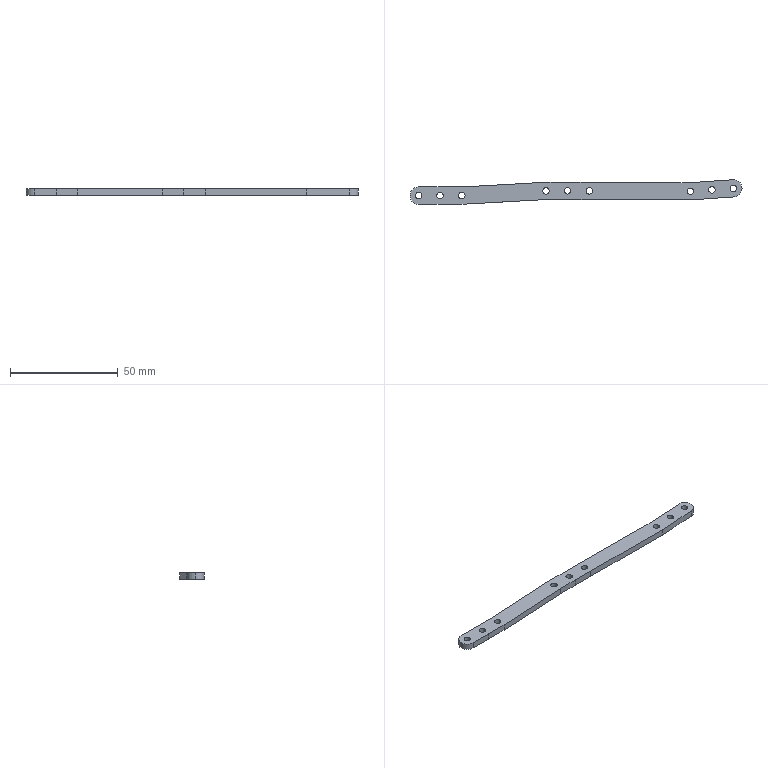Part | SolidWorks | features Extrusion 1 | 1 solid | 37 faces | box 153.919 x 11.375 x 3 mm | volume 3465 mm3 | cylinder 21 | plane 16 | commonest cylinder face diameters 3 x18 8 x3
STEP:
#1=CARTESIAN_POINT('',(75.386,1.147,3.));
#2=VERTEX_POINT('',#1);
#3=CARTESIAN_POINT('',(78.386,1.147,3.));
#4=VERTEX_POINT('',#3);
#5=CARTESIAN_POINT('',(76.886,1.147,3.));
#6=DIRECTION('',(0.,0.,1.));
#7=DIRECTION('',(1.,0.,0.));
#8=AXIS2_PLACEMENT_3D('',#5,#6,#7);
#9=CIRCLE('',#8,1.5);
#10=EDGE_CURVE('',#2,#4,#9,.T.);
#11=ORIENTED_EDGE('',*,*,#10,.T.);
#12=CARTESIAN_POINT('',(78.386,1.147,0.));
#13=VERTEX_POINT('',#12);
#14=CARTESIAN_POINT('',(78.386,1.147,3.));
#15=DIRECTION('',(0.,0.,-1.));
#16=VECTOR('',#15,1000.);
#17=LINE('',#14,#16);
#18=EDGE_CURVE('',#4,#13,#17,.T.);
#19=ORIENTED_EDGE('',*,*,#18,.T.);
#20=CARTESIAN_POINT('',(75.386,1.147,0.));
#21=VERTEX_POINT('',#20);
#22=CARTESIAN_POINT('',(76.886,1.147,0.));
#23=DIRECTION('',(0.,0.,1.));
#24=DIRECTION('',(1.,0.,0.));
#25=AXIS2_PLACEMENT_3D('',#22,#23,#24);
#26=CIRCLE('',#25,1.5);
#27=EDGE_CURVE('',#21,#13,#26,.T.);
#28=ORIENTED_EDGE('',*,*,#27,.F.);
#29=CARTESIAN_POINT('',(75.386,1.147,3.));
#30=DIRECTION('',(0.,0.,-1.));
#31=VECTOR('',#30,1000.);
#32=LINE('',#29,#31);
#33=EDGE_CURVE('',#2,#21,#32,.T.);
#34=ORIENTED_EDGE('',*,*,#33,.F.);
#35=EDGE_LOOP('',(#11,#19,#28,#34));
#36=FACE_OUTER_BOUND('',#35,.T.);
#37=CARTESIAN_POINT('',(76.886,1.147,3.));
#38=DIRECTION('',(0.,0.,-1.));
#39=DIRECTION('',(-1.,0.,0.));
#40=AXIS2_PLACEMENT_3D('',#37,#38,#39);
#41=CYLINDRICAL_SURFACE('',#40,1.5);
#42=ADVANCED_FACE('',(#36),#41,.F.);
#43=CARTESIAN_POINT('',(65.409,0.4705,3.));
#44=VERTEX_POINT('',#43);
#45=CARTESIAN_POINT('',(68.409,0.4705,3.));
#46=VERTEX_POINT('',#45);
#47=CARTESIAN_POINT('',(66.909,0.4705,3.));
#48=DIRECTION('',(0.,0.,1.));
#49=DIRECTION('',(1.,0.,0.));
#50=AXIS2_PLACEMENT_3D('',#47,#48,#49);
#51=CIRCLE('',#50,1.5);
#52=EDGE_CURVE('',#44,#46,#51,.T.);
#53=ORIENTED_EDGE('',*,*,#52,.T.);
#54=CARTESIAN_POINT('',(68.409,0.4705,0.));
#55=VERTEX_POINT('',#54);
#56=CARTESIAN_POINT('',(68.409,0.4705,3.));
#57=DIRECTION('',(0.,0.,-1.));
#58=VECTOR('',#57,1000.);
#59=LINE('',#56,#58);
#60=EDGE_CURVE('',#46,#55,#59,.T.);
#61=ORIENTED_EDGE('',*,*,#60,.T.);
#62=CARTESIAN_POINT('',(65.409,0.4705,0.));
#63=VERTEX_POINT('',#62);
#64=CARTESIAN_POINT('',(66.909,0.4705,0.));
#65=DIRECTION('',(0.,0.,1.));
#66=DIRECTION('',(1.,0.,0.));
#67=AXIS2_PLACEMENT_3D('',#64,#65,#66);
#68=CIRCLE('',#67,1.5);
#69=EDGE_CURVE('',#63,#55,#68,.T.);
#70=ORIENTED_EDGE('',*,*,#69,.F.);
#71=CARTESIAN_POINT('',(65.409,0.4705,3.));
#72=DIRECTION('',(0.,0.,-1.));
#73=VECTOR('',#72,1000.);
#74=LINE('',#71,#73);
#75=EDGE_CURVE('',#44,#63,#74,.T.);
#76=ORIENTED_EDGE('',*,*,#75,.F.);
#77=EDGE_LOOP('',(#53,#61,#70,#76));
#78=FACE_OUTER_BOUND('',#77,.T.);
#79=CARTESIAN_POINT('',(66.909,0.4705,3.));
#80=DIRECTION('',(0.,0.,-1.));
#81=DIRECTION('',(-1.,0.,0.));
#82=AXIS2_PLACEMENT_3D('',#79,#80,#81);
#83=CYLINDRICAL_SURFACE('',#82,1.5);
#84=ADVANCED_FACE('',(#78),#83,.F.);
#85=CARTESIAN_POINT('',(55.432,-0.2061,3.));
#86=VERTEX_POINT('',#85);
#87=CARTESIAN_POINT('',(58.432,-0.2061,3.));
#88=VERTEX_POINT('',#87);
#89=CARTESIAN_POINT('',(56.932,-0.2061,3.));
#90=DIRECTION('',(0.,0.,1.));
#91=DIRECTION('',(1.,0.,0.));
#92=AXIS2_PLACEMENT_3D('',#89,#90,#91);
#93=CIRCLE('',#92,1.5);
#94=EDGE_CURVE('',#86,#88,#93,.T.);
#95=ORIENTED_EDGE('',*,*,#94,.T.);
#96=CARTESIAN_POINT('',(58.432,-0.2061,0.));
#97=VERTEX_POINT('',#96);
#98=CARTESIAN_POINT('',(58.432,-0.2061,3.));
#99=DIRECTION('',(0.,0.,-1.));
#100=VECTOR('',#99,1000.);
#101=LINE('',#98,#100);
#102=EDGE_CURVE('',#88,#97,#101,.T.);
#103=ORIENTED_EDGE('',*,*,#102,.T.);
#104=CARTESIAN_POINT('',(55.432,-0.2061,0.));
#105=VERTEX_POINT('',#104);
#106=CARTESIAN_POINT('',(56.932,-0.2061,0.));
#107=DIRECTION('',(0.,0.,1.));
#108=DIRECTION('',(1.,0.,0.));
#109=AXIS2_PLACEMENT_3D('',#106,#107,#108);
#110=CIRCLE('',#109,1.5);
#111=EDGE_CURVE('',#105,#97,#110,.T.);
#112=ORIENTED_EDGE('',*,*,#111,.F.);
#113=CARTESIAN_POINT('',(55.432,-0.2061,3.));
#114=DIRECTION('',(0.,0.,-1.));
#115=VECTOR('',#114,1000.);
#116=LINE('',#113,#115);
#117=EDGE_CURVE('',#86,#105,#116,.T.);
#118=ORIENTED_EDGE('',*,*,#117,.F.);
#119=EDGE_LOOP('',(#95,#103,#112,#118));
#120=FACE_OUTER_BOUND('',#119,.T.);
#121=CARTESIAN_POINT('',(56.932,-0.2061,3.));
#122=DIRECTION('',(0.,0.,-1.));
#123=DIRECTION('',(-1.,0.,0.));
#124=AXIS2_PLACEMENT_3D('',#121,#122,#123);
#125=CYLINDRICAL_SURFACE('',#124,1.5);
#126=ADVANCED_FACE('',(#120),#125,.F.);
#127=CARTESIAN_POINT('',(8.574,-0.03311,3.));
#128=VERTEX_POINT('',#127);
#129=CARTESIAN_POINT('',(11.574,-0.03311,3.));
#130=VERTEX_POINT('',#129);
#131=CARTESIAN_POINT('',(10.074,-0.03311,3.));
#132=DIRECTION('',(0.,0.,1.));
#133=DIRECTION('',(1.,0.,0.));
#134=AXIS2_PLACEMENT_3D('',#131,#132,#133);
#135=CIRCLE('',#134,1.5);
#136=EDGE_CURVE('',#128,#130,#135,.T.);
#137=ORIENTED_EDGE('',*,*,#136,.T.);
#138=CARTESIAN_POINT('',(11.574,-0.03311,0.));
#139=VERTEX_POINT('',#138);
#140=CARTESIAN_POINT('',(11.574,-0.03311,3.));
#141=DIRECTION('',(0.,0.,-1.));
#142=VECTOR('',#141,1000.);
#143=LINE('',#140,#142);
#144=EDGE_CURVE('',#130,#139,#143,.T.);
#145=ORIENTED_EDGE('',*,*,#144,.T.);
#146=CARTESIAN_POINT('',(8.574,-0.03311,0.));
#147=VERTEX_POINT('',#146);
#148=CARTESIAN_POINT('',(10.074,-0.03311,0.));
#149=DIRECTION('',(0.,0.,1.));
#150=DIRECTION('',(1.,0.,0.));
#151=AXIS2_PLACEMENT_3D('',#148,#149,#150);
#152=CIRCLE('',#151,1.5);
#153=EDGE_CURVE('',#147,#139,#152,.T.);
#154=ORIENTED_EDGE('',*,*,#153,.F.);
#155=CARTESIAN_POINT('',(8.574,-0.03311,3.));
#156=DIRECTION('',(0.,0.,-1.));
#157=VECTOR('',#156,1000.);
#158=LINE('',#155,#157);
#159=EDGE_CURVE('',#128,#147,#158,.T.);
#160=ORIENTED_EDGE('',*,*,#159,.F.);
#161=EDGE_LOOP('',(#137,#145,#154,#160));
#162=FACE_OUTER_BOUND('',#161,.T.);
#163=CARTESIAN_POINT('',(10.074,-0.03311,3.));
#164=DIRECTION('',(0.,0.,-1.));
#165=DIRECTION('',(-1.,0.,0.));
#166=AXIS2_PLACEMENT_3D('',#163,#164,#165);
#167=CYLINDRICAL_SURFACE('',#166,1.5);
#168=ADVANCED_FACE('',(#162),#167,.F.);
#169=CARTESIAN_POINT('',(-1.5,0.,3.));
#170=VERTEX_POINT('',#169);
#171=CARTESIAN_POINT('',(1.5,0.,3.));
#172=VERTEX_POINT('',#171);
#173=CARTESIAN_POINT('',(0.,0.,3.));
#174=DIRECTION('',(0.,0.,1.));
#175=DIRECTION('',(1.,0.,0.));
#176=AXIS2_PLACEMENT_3D('',#173,#174,#175);
#177=CIRCLE('',#176,1.5);
#178=EDGE_CURVE('',#170,#172,#177,.T.);
#179=ORIENTED_EDGE('',*,*,#178,.T.);
#180=CARTESIAN_POINT('',(1.5,0.,0.));
#181=VERTEX_POINT('',#180);
#182=CARTESIAN_POINT('',(1.5,0.,3.));
#183=DIRECTION('',(0.,0.,-1.));
#184=VECTOR('',#183,1000.);
#185=LINE('',#182,#184);
#186=EDGE_CURVE('',#172,#181,#185,.T.);
#187=ORIENTED_EDGE('',*,*,#186,.T.);
#188=CARTESIAN_POINT('',(-1.5,0.,0.));
#189=VERTEX_POINT('',#188);
#190=CARTESIAN_POINT('',(0.,0.,0.));
#191=DIRECTION('',(0.,0.,1.));
#192=DIRECTION('',(1.,0.,0.));
#193=AXIS2_PLACEMENT_3D('',#190,#191,#192);
#194=CIRCLE('',#193,1.5);
#195=EDGE_CURVE('',#189,#181,#194,.T.);
#196=ORIENTED_EDGE('',*,*,#195,.F.);
#197=CARTESIAN_POINT('',(-1.5,0.,3.));
#198=DIRECTION('',(0.,0.,-1.));
#199=VECTOR('',#198,1000.);
#200=LINE('',#197,#199);
#201=EDGE_CURVE('',#170,#189,#200,.T.);
#202=ORIENTED_EDGE('',*,*,#201,.F.);
#203=EDGE_LOOP('',(#179,#187,#196,#202));
#204=FACE_OUTER_BOUND('',#203,.T.);
#205=CARTESIAN_POINT('',(0.,0.,3.));
#206=DIRECTION('',(0.,0.,-1.));
#207=DIRECTION('',(-1.,0.,0.));
#208=AXIS2_PLACEMENT_3D('',#205,#206,#207);
#209=CYLINDRICAL_SURFACE('',#208,1.5);
#210=ADVANCED_FACE('',(#204),#209,.F.);
#211=CARTESIAN_POINT('',(-70.532,-2.227,3.));
#212=VERTEX_POINT('',#211);
#213=CARTESIAN_POINT('',(-67.532,-2.227,3.));
#214=VERTEX_POINT('',#213);
#215=CARTESIAN_POINT('',(-69.032,-2.227,3.));
#216=DIRECTION('',(0.,0.,1.));
#217=DIRECTION('',(1.,0.,0.));
#218=AXIS2_PLACEMENT_3D('',#215,#216,#217);
#219=CIRCLE('',#218,1.5);
#220=EDGE_CURVE('',#212,#214,#219,.T.);
#221=ORIENTED_EDGE('',*,*,#220,.T.);
#222=CARTESIAN_POINT('',(-67.532,-2.227,0.));
#223=VERTEX_POINT('',#222);
#224=CARTESIAN_POINT('',(-67.532,-2.227,3.));
#225=DIRECTION('',(0.,0.,-1.));
#226=VECTOR('',#225,1000.);
#227=LINE('',#224,#226);
#228=EDGE_CURVE('',#214,#223,#227,.T.);
#229=ORIENTED_EDGE('',*,*,#228,.T.);
#230=CARTESIAN_POINT('',(-70.532,-2.227,0.));
#231=VERTEX_POINT('',#230);
#232=CARTESIAN_POINT('',(-69.032,-2.227,0.));
#233=DIRECTION('',(0.,0.,1.));
#234=DIRECTION('',(1.,0.,0.));
#235=AXIS2_PLACEMENT_3D('',#232,#233,#234);
#236=CIRCLE('',#235,1.5);
#237=EDGE_CURVE('',#231,#223,#236,.T.);
#238=ORIENTED_EDGE('',*,*,#237,.F.);
#239=CARTESIAN_POINT('',(-70.532,-2.227,3.));
#240=DIRECTION('',(0.,0.,-1.));
#241=VECTOR('',#240,1000.);
#242=LINE('',#239,#241);
#243=EDGE_CURVE('',#212,#231,#242,.T.);
#244=ORIENTED_EDGE('',*,*,#243,.F.);
#245=EDGE_LOOP('',(#221,#229,#238,#244));
#246=FACE_OUTER_BOUND('',#245,.T.);
#247=CARTESIAN_POINT('',(-69.032,-2.227,3.));
#248=DIRECTION('',(0.,0.,-1.));
#249=DIRECTION('',(-1.,0.,0.));
#250=AXIS2_PLACEMENT_3D('',#247,#248,#249);
#251=CYLINDRICAL_SURFACE('',#250,1.5);
#252=ADVANCED_FACE('',(#246),#251,.F.);
#253=CARTESIAN_POINT('',(-11.426,-0.03311,3.));
#254=VERTEX_POINT('',#253);
#255=CARTESIAN_POINT('',(-8.426,-0.03311,3.));
#256=VERTEX_POINT('',#255);
#257=CARTESIAN_POINT('',(-9.926,-0.03311,3.));
#258=DIRECTION('',(0.,0.,1.));
#259=DIRECTION('',(1.,0.,0.));
#260=AXIS2_PLACEMENT_3D('',#257,#258,#259);
#261=CIRCLE('',#260,1.5);
#262=EDGE_CURVE('',#254,#256,#261,.T.);
#263=ORIENTED_EDGE('',*,*,#262,.T.);
#264=CARTESIAN_POINT('',(-8.426,-0.03311,0.));
#265=VERTEX_POINT('',#264);
#266=CARTESIAN_POINT('',(-8.426,-0.03311,3.));
#267=DIRECTION('',(0.,0.,-1.));
#268=VECTOR('',#267,1000.);
#269=LINE('',#266,#268);
#270=EDGE_CURVE('',#256,#265,#269,.T.);
#271=ORIENTED_EDGE('',*,*,#270,.T.);
#272=CARTESIAN_POINT('',(-11.426,-0.03311,0.));
#273=VERTEX_POINT('',#272);
#274=CARTESIAN_POINT('',(-9.926,-0.03311,0.));
#275=DIRECTION('',(0.,0.,1.));
#276=DIRECTION('',(1.,0.,0.));
#277=AXIS2_PLACEMENT_3D('',#274,#275,#276);
#278=CIRCLE('',#277,1.5);
#279=EDGE_CURVE('',#273,#265,#278,.T.);
#280=ORIENTED_EDGE('',*,*,#279,.F.);
#281=CARTESIAN_POINT('',(-11.426,-0.03311,3.));
#282=DIRECTION('',(0.,0.,-1.));
#283=VECTOR('',#282,1000.);
#284=LINE('',#281,#283);
#285=EDGE_CURVE('',#254,#273,#284,.T.);
#286=ORIENTED_EDGE('',*,*,#285,.F.);
#287=EDGE_LOOP('',(#263,#271,#280,#286));
#288=FACE_OUTER_BOUND('',#287,.T.);
#289=CARTESIAN_POINT('',(-9.926,-0.03311,3.));
#290=DIRECTION('',(0.,0.,-1.));
#291=DIRECTION('',(-1.,0.,0.));
#292=AXIS2_PLACEMENT_3D('',#289,#290,#291);
#293=CYLINDRICAL_SURFACE('',#292,1.5);
#294=ADVANCED_FACE('',(#288),#293,.F.);
#295=CARTESIAN_POINT('',(-50.532,-2.227,3.));
#296=VERTEX_POINT('',#295);
#297=CARTESIAN_POINT('',(-47.532,-2.227,3.));
#298=VERTEX_POINT('',#297);
#299=CARTESIAN_POINT('',(-49.032,-2.227,3.));
#300=DIRECTION('',(0.,0.,1.));
#301=DIRECTION('',(1.,0.,0.));
#302=AXIS2_PLACEMENT_3D('',#299,#300,#301);
#303=CIRCLE('',#302,1.5);
#304=EDGE_CURVE('',#296,#298,#303,.T.);
#305=ORIENTED_EDGE('',*,*,#304,.T.);
#306=CARTESIAN_POINT('',(-47.532,-2.227,0.));
#307=VERTEX_POINT('',#306);
#308=CARTESIAN_POINT('',(-47.532,-2.227,3.));
#309=DIRECTION('',(0.,0.,-1.));
#310=VECTOR('',#309,1000.);
#311=LINE('',#308,#310);
#312=EDGE_CURVE('',#298,#307,#311,.T.);
#313=ORIENTED_EDGE('',*,*,#312,.T.);
#314=CARTESIAN_POINT('',(-50.532,-2.227,0.));
#315=VERTEX_POINT('',#314);
#316=CARTESIAN_POINT('',(-49.032,-2.227,0.));
#317=DIRECTION('',(0.,0.,1.));
#318=DIRECTION('',(1.,0.,0.));
#319=AXIS2_PLACEMENT_3D('',#316,#317,#318);
#320=CIRCLE('',#319,1.5);
#321=EDGE_CURVE('',#315,#307,#320,.T.);
#322=ORIENTED_EDGE('',*,*,#321,.F.);
#323=CARTESIAN_POINT('',(-50.532,-2.227,3.));
#324=DIRECTION('',(0.,0.,-1.));
#325=VECTOR('',#324,1000.);
#326=LINE('',#323,#325);
#327=EDGE_CURVE('',#296,#315,#326,.T.);
#328=ORIENTED_EDGE('',*,*,#327,.F.);
#329=EDGE_LOOP('',(#305,#313,#322,#328));
#330=FACE_OUTER_BOUND('',#329,.T.);
#331=CARTESIAN_POINT('',(-49.032,-2.227,3.));
#332=DIRECTION('',(0.,0.,-1.));
#333=DIRECTION('',(-1.,0.,0.));
#334=AXIS2_PLACEMENT_3D('',#331,#332,#333);
#335=CYLINDRICAL_SURFACE('',#334,1.5);
#336=ADVANCED_FACE('',(#330),#335,.F.);
#337=CARTESIAN_POINT('',(-60.602,-2.196,3.));
#338=VERTEX_POINT('',#337);
#339=CARTESIAN_POINT('',(-57.602,-2.196,3.));
#340=VERTEX_POINT('',#339);
#341=CARTESIAN_POINT('',(-59.102,-2.196,3.));
#342=DIRECTION('',(0.,0.,1.));
#343=DIRECTION('',(1.,0.,0.));
#344=AXIS2_PLACEMENT_3D('',#341,#342,#343);
#345=CIRCLE('',#344,1.5);
#346=EDGE_CURVE('',#338,#340,#345,.T.);
#347=ORIENTED_EDGE('',*,*,#346,.T.);
#348=CARTESIAN_POINT('',(-57.602,-2.196,0.));
#349=VERTEX_POINT('',#348);
#350=CARTESIAN_POINT('',(-57.602,-2.196,3.));
#351=DIRECTION('',(0.,0.,-1.));
#352=VECTOR('',#351,1000.);
#353=LINE('',#350,#352);
#354=EDGE_CURVE('',#340,#349,#353,.T.);
#355=ORIENTED_EDGE('',*,*,#354,.T.);
#356=CARTESIAN_POINT('',(-60.602,-2.196,0.));
#357=VERTEX_POINT('',#356);
#358=CARTESIAN_POINT('',(-59.102,-2.196,0.));
#359=DIRECTION('',(0.,0.,1.));
#360=DIRECTION('',(1.,0.,0.));
#361=AXIS2_PLACEMENT_3D('',#358,#359,#360);
#362=CIRCLE('',#361,1.5);
#363=EDGE_CURVE('',#357,#349,#362,.T.);
#364=ORIENTED_EDGE('',*,*,#363,.F.);
#365=CARTESIAN_POINT('',(-60.602,-2.196,3.));
#366=DIRECTION('',(0.,0.,-1.));
#367=VECTOR('',#366,1000.);
#368=LINE('',#365,#367);
#369=EDGE_CURVE('',#338,#357,#368,.T.);
#370=ORIENTED_EDGE('',*,*,#369,.F.);
#371=EDGE_LOOP('',(#347,#355,#364,#370));
#372=FACE_OUTER_BOUND('',#371,.T.);
#373=CARTESIAN_POINT('',(-59.102,-2.196,3.));
#374=DIRECTION('',(0.,0.,-1.));
#375=DIRECTION('',(-1.,0.,0.));
#376=AXIS2_PLACEMENT_3D('',#373,#374,#375);
#377=CYLINDRICAL_SURFACE('',#376,1.5);
#378=ADVANCED_FACE('',(#372),#377,.F.);
#379=CARTESIAN_POINT('',(-73.032,-2.227,3.));
#380=VERTEX_POINT('',#379);
#381=CARTESIAN_POINT('',(-69.02,-6.227,3.));
#382=VERTEX_POINT('',#381);
#383=CARTESIAN_POINT('',(-69.032,-2.227,3.));
#384=DIRECTION('',(0.,0.,1.));
#385=DIRECTION('',(1.,0.,0.));
#386=AXIS2_PLACEMENT_3D('',#383,#384,#385);
#387=CIRCLE('',#386,4.);
#388=EDGE_CURVE('',#380,#382,#387,.T.);
#389=ORIENTED_EDGE('',*,*,#388,.F.);
#390=CARTESIAN_POINT('',(-73.032,-2.227,0.));
#391=VERTEX_POINT('',#390);
#392=CARTESIAN_POINT('',(-73.032,-2.227,3.));
#393=DIRECTION('',(0.,0.,-1.));
#394=VECTOR('',#393,1000.);
#395=LINE('',#392,#394);
#396=EDGE_CURVE('',#380,#391,#395,.T.);
#397=ORIENTED_EDGE('',*,*,#396,.T.);
#398=CARTESIAN_POINT('',(-69.02,-6.227,0.));
#399=VERTEX_POINT('',#398);
#400=CARTESIAN_POINT('',(-69.032,-2.227,0.));
#401=DIRECTION('',(0.,0.,1.));
#402=DIRECTION('',(1.,0.,0.));
#403=AXIS2_PLACEMENT_3D('',#400,#401,#402);
#404=CIRCLE('',#403,4.);
#405=EDGE_CURVE('',#391,#399,#404,.T.);
#406=ORIENTED_EDGE('',*,*,#405,.T.);
#407=CARTESIAN_POINT('',(-69.02,-6.227,3.));
#408=DIRECTION('',(0.,0.,-1.));
#409=VECTOR('',#408,1000.);
#410=LINE('',#407,#409);
#411=EDGE_CURVE('',#382,#399,#410,.T.);
#412=ORIENTED_EDGE('',*,*,#411,.F.);
#413=EDGE_LOOP('',(#389,#397,#406,#412));
#414=FACE_OUTER_BOUND('',#413,.T.);
#415=CARTESIAN_POINT('',(-69.032,-2.227,3.));
#416=DIRECTION('',(0.,0.,-1.));
#417=DIRECTION('',(-1.,0.,0.));
#418=AXIS2_PLACEMENT_3D('',#415,#416,#417);
#419=CYLINDRICAL_SURFACE('',#418,4.);
#420=ADVANCED_FACE('',(#414),#419,.T.);
#421=ORIENTED_EDGE('',*,*,#52,.F.);
#422=CARTESIAN_POINT('',(66.909,0.4705,3.));
#423=DIRECTION('',(0.,0.,1.));
#424=DIRECTION('',(1.,0.,0.));
#425=AXIS2_PLACEMENT_3D('',#422,#423,#424);
#426=CIRCLE('',#425,1.5);
#427=EDGE_CURVE('',#46,#44,#426,.T.);
#428=ORIENTED_EDGE('',*,*,#427,.F.);
#429=EDGE_LOOP('',(#421,#428));
#430=FACE_BOUND('',#429,.T.);
#431=ORIENTED_EDGE('',*,*,#136,.F.);
#432=CARTESIAN_POINT('',(10.074,-0.03311,3.));
#433=DIRECTION('',(0.,0.,1.));
#434=DIRECTION('',(1.,0.,0.));
#435=AXIS2_PLACEMENT_3D('',#432,#433,#434);
#436=CIRCLE('',#435,1.5);
#437=EDGE_CURVE('',#130,#128,#436,.T.);
#438=ORIENTED_EDGE('',*,*,#437,.F.);
#439=EDGE_LOOP('',(#431,#438));
#440=FACE_BOUND('',#439,.T.);
#441=ORIENTED_EDGE('',*,*,#220,.F.);
#442=CARTESIAN_POINT('',(-69.032,-2.227,3.));
#443=DIRECTION('',(0.,0.,1.));
#444=DIRECTION('',(1.,0.,0.));
#445=AXIS2_PLACEMENT_3D('',#442,#443,#444);
#446=CIRCLE('',#445,1.5);
#447=EDGE_CURVE('',#214,#212,#446,.T.);
#448=ORIENTED_EDGE('',*,*,#447,.F.);
#449=EDGE_LOOP('',(#441,#448));
#450=FACE_BOUND('',#449,.T.);
#451=ORIENTED_EDGE('',*,*,#304,.F.);
#452=CARTESIAN_POINT('',(-49.032,-2.227,3.));
#453=DIRECTION('',(0.,0.,1.));
#454=DIRECTION('',(1.,0.,0.));
#455=AXIS2_PLACEMENT_3D('',#452,#453,#454);
#456=CIRCLE('',#455,1.5);
#457=EDGE_CURVE('',#298,#296,#456,.T.);
#458=ORIENTED_EDGE('',*,*,#457,.F.);
#459=EDGE_LOOP('',(#451,#458));
#460=FACE_BOUND('',#459,.T.);
#461=CARTESIAN_POINT('',(-69.045,1.773,3.));
#462=VERTEX_POINT('',#461);
#463=CARTESIAN_POINT('',(-69.032,-2.227,3.));
#464=DIRECTION('',(0.,0.,1.));
#465=DIRECTION('',(1.,0.,0.));
#466=AXIS2_PLACEMENT_3D('',#463,#464,#465);
#467=CIRCLE('',#466,4.);
#468=EDGE_CURVE('',#462,#380,#467,.T.);
#469=ORIENTED_EDGE('',*,*,#468,.T.);
#470=ORIENTED_EDGE('',*,*,#388,.T.);
#471=CARTESIAN_POINT('',(-59.102,-6.196,3.));
#472=VERTEX_POINT('',#471);
#473=CARTESIAN_POINT('',(-69.02,-6.227,3.));
#474=DIRECTION('',(1.,0.003128,0.));
#475=VECTOR('',#474,1000.);
#476=LINE('',#473,#475);
#477=EDGE_CURVE('',#382,#472,#476,.T.);
#478=ORIENTED_EDGE('',*,*,#477,.T.);
#479=CARTESIAN_POINT('',(-48.926,-6.228,3.));
#480=VERTEX_POINT('',#479);
#481=CARTESIAN_POINT('',(-59.102,-6.196,3.));
#482=DIRECTION('',(1.,-0.003085,0.));
#483=VECTOR('',#482,1000.);
#484=LINE('',#481,#483);
#485=EDGE_CURVE('',#472,#480,#484,.T.);
#486=ORIENTED_EDGE('',*,*,#485,.T.);
#487=CARTESIAN_POINT('',(-9.807,-4.033,3.));
#488=VERTEX_POINT('',#487);
#489=CARTESIAN_POINT('',(-48.926,-6.228,3.));
#490=DIRECTION('',(0.9984,0.05602,0.));
#491=VECTOR('',#490,1000.);
#492=LINE('',#489,#491);
#493=EDGE_CURVE('',#480,#488,#492,.T.);
#494=ORIENTED_EDGE('',*,*,#493,.T.);
#495=CARTESIAN_POINT('',(0.0000982,-4.,3.));
#496=VERTEX_POINT('',#495);
#497=CARTESIAN_POINT('',(-9.807,-4.033,3.));
#498=DIRECTION('',(1.,0.003335,0.));
#499=VECTOR('',#498,1000.);
#500=LINE('',#497,#499);
#501=EDGE_CURVE('',#488,#496,#500,.T.);
#502=ORIENTED_EDGE('',*,*,#501,.T.);
#503=CARTESIAN_POINT('',(10.06,-4.033,3.));
#504=VERTEX_POINT('',#503);
#505=CARTESIAN_POINT('',(0.0000982,-4.,3.));
#506=DIRECTION('',(1.,-0.003286,0.));
#507=VECTOR('',#506,1000.);
#508=LINE('',#505,#507);
#509=EDGE_CURVE('',#496,#504,#508,.T.);
#510=ORIENTED_EDGE('',*,*,#509,.T.);
#511=CARTESIAN_POINT('',(57.06,-4.207,3.));
#512=VERTEX_POINT('',#511);
#513=CARTESIAN_POINT('',(10.06,-4.033,3.));
#514=DIRECTION('',(1.,-0.003691,0.));
#515=VECTOR('',#514,1000.);
#516=LINE('',#513,#515);
#517=EDGE_CURVE('',#504,#512,#516,.T.);
#518=ORIENTED_EDGE('',*,*,#517,.T.);
#519=CARTESIAN_POINT('',(77.157,-2.844,3.));
#520=VERTEX_POINT('',#519);
#521=CARTESIAN_POINT('',(57.06,-4.207,3.));
#522=DIRECTION('',(0.9977,0.06765,0.));
#523=VECTOR('',#522,1000.);
#524=LINE('',#521,#523);
#525=EDGE_CURVE('',#512,#520,#524,.T.);
#526=ORIENTED_EDGE('',*,*,#525,.T.);
#527=CARTESIAN_POINT('',(76.616,5.138,3.));
#528=VERTEX_POINT('',#527);
#529=CARTESIAN_POINT('',(76.886,1.147,3.));
#530=DIRECTION('',(0.,0.,1.));
#531=DIRECTION('',(1.,0.,0.));
#532=AXIS2_PLACEMENT_3D('',#529,#530,#531);
#533=CIRCLE('',#532,4.);
#534=EDGE_CURVE('',#520,#528,#533,.T.);
#535=ORIENTED_EDGE('',*,*,#534,.T.);
#536=CARTESIAN_POINT('',(56.804,3.794,3.));
#537=VERTEX_POINT('',#536);
#538=CARTESIAN_POINT('',(66.639,4.461,3.));
#539=DIRECTION('',(-0.9977,-0.06765,0.));
#540=VECTOR('',#539,1000.);
#541=LINE('',#538,#540);
#542=EDGE_CURVE('',#528,#537,#541,.T.);
#543=ORIENTED_EDGE('',*,*,#542,.T.);
#544=CARTESIAN_POINT('',(10.088,3.967,3.));
#545=VERTEX_POINT('',#544);
#546=CARTESIAN_POINT('',(10.088,3.967,3.));
#547=DIRECTION('',(-1.,0.003691,0.));
#548=VECTOR('',#547,1000.);
#549=LINE('',#546,#548);
#550=EDGE_CURVE('',#537,#545,#549,.T.);
#551=ORIENTED_EDGE('',*,*,#550,.T.);
#552=CARTESIAN_POINT('',(-0.0000982,4.,3.));
#553=VERTEX_POINT('',#552);
#554=CARTESIAN_POINT('',(-0.0000982,4.,3.));
#555=DIRECTION('',(-1.,0.003286,0.));
#556=VECTOR('',#555,1000.);
#557=LINE('',#554,#556);
#558=EDGE_CURVE('',#545,#553,#557,.T.);
#559=ORIENTED_EDGE('',*,*,#558,.T.);
#560=CARTESIAN_POINT('',(-10.045,3.967,3.));
#561=VERTEX_POINT('',#560);
#562=CARTESIAN_POINT('',(-10.045,3.967,3.));
#563=DIRECTION('',(-1.,-0.003335,0.));
#564=VECTOR('',#563,1000.);
#565=LINE('',#562,#564);
#566=EDGE_CURVE('',#553,#561,#565,.T.);
#567=ORIENTED_EDGE('',*,*,#566,.T.);
#568=CARTESIAN_POINT('',(-49.138,1.773,3.));
#569=VERTEX_POINT('',#568);
#570=CARTESIAN_POINT('',(-49.138,1.773,3.));
#571=DIRECTION('',(-0.9984,-0.05602,0.));
#572=VECTOR('',#571,1000.);
#573=LINE('',#570,#572);
#574=EDGE_CURVE('',#561,#569,#573,.T.);
#575=ORIENTED_EDGE('',*,*,#574,.T.);
#576=CARTESIAN_POINT('',(-59.102,1.804,3.));
#577=VERTEX_POINT('',#576);
#578=CARTESIAN_POINT('',(-59.102,1.804,3.));
#579=DIRECTION('',(-1.,0.003085,0.));
#580=VECTOR('',#579,1000.);
#581=LINE('',#578,#580);
#582=EDGE_CURVE('',#569,#577,#581,.T.);
#583=ORIENTED_EDGE('',*,*,#582,.T.);
#584=CARTESIAN_POINT('',(-69.045,1.773,3.));
#585=DIRECTION('',(-1.,-0.003128,0.));
#586=VECTOR('',#585,1000.);
#587=LINE('',#584,#586);
#588=EDGE_CURVE('',#577,#462,#587,.T.);
#589=ORIENTED_EDGE('',*,*,#588,.T.);
#590=EDGE_LOOP('',(#469,#470,#478,#486,#494,#502,#510,#518,#526,#535,#543,#551,#559,#567,#575,#583,#589));
#591=FACE_OUTER_BOUND('',#590,.T.);
#592=ORIENTED_EDGE('',*,*,#346,.F.);
#593=CARTESIAN_POINT('',(-59.102,-2.196,3.));
#594=DIRECTION('',(0.,0.,1.));
#595=DIRECTION('',(1.,0.,0.));
#596=AXIS2_PLACEMENT_3D('',#593,#594,#595);
#597=CIRCLE('',#596,1.5);
#598=EDGE_CURVE('',#340,#338,#597,.T.);
#599=ORIENTED_EDGE('',*,*,#598,.F.);
#600=EDGE_LOOP('',(#592,#599));
#601=FACE_BOUND('',#600,.T.);
#602=ORIENTED_EDGE('',*,*,#262,.F.);
#603=CARTESIAN_POINT('',(-9.926,-0.03311,3.));
#604=DIRECTION('',(0.,0.,1.));
#605=DIRECTION('',(1.,0.,0.));
#606=AXIS2_PLACEMENT_3D('',#603,#604,#605);
#607=CIRCLE('',#606,1.5);
#608=EDGE_CURVE('',#256,#254,#607,.T.);
#609=ORIENTED_EDGE('',*,*,#608,.F.);
#610=EDGE_LOOP('',(#602,#609));
#611=FACE_BOUND('',#610,.T.);
#612=ORIENTED_EDGE('',*,*,#178,.F.);
#613=CARTESIAN_POINT('',(0.,0.,3.));
#614=DIRECTION('',(0.,0.,1.));
#615=DIRECTION('',(1.,0.,0.));
#616=AXIS2_PLACEMENT_3D('',#613,#614,#615);
#617=CIRCLE('',#616,1.5);
#618=EDGE_CURVE('',#172,#170,#617,.T.);
#619=ORIENTED_EDGE('',*,*,#618,.F.);
#620=EDGE_LOOP('',(#612,#619));
#621=FACE_BOUND('',#620,.T.);
#622=ORIENTED_EDGE('',*,*,#94,.F.);
#623=CARTESIAN_POINT('',(56.932,-0.2061,3.));
#624=DIRECTION('',(0.,0.,1.));
#625=DIRECTION('',(1.,0.,0.));
#626=AXIS2_PLACEMENT_3D('',#623,#624,#625);
#627=CIRCLE('',#626,1.5);
#628=EDGE_CURVE('',#88,#86,#627,.T.);
#629=ORIENTED_EDGE('',*,*,#628,.F.);
#630=EDGE_LOOP('',(#622,#629));
#631=FACE_BOUND('',#630,.T.);
#632=ORIENTED_EDGE('',*,*,#10,.F.);
#633=CARTESIAN_POINT('',(76.886,1.147,3.));
#634=DIRECTION('',(0.,0.,1.));
#635=DIRECTION('',(1.,0.,0.));
#636=AXIS2_PLACEMENT_3D('',#633,#634,#635);
#637=CIRCLE('',#636,1.5);
#638=EDGE_CURVE('',#4,#2,#637,.T.);
#639=ORIENTED_EDGE('',*,*,#638,.F.);
#640=EDGE_LOOP('',(#632,#639));
#641=FACE_BOUND('',#640,.T.);
#642=CARTESIAN_POINT('',(-69.032,-2.227,3.));
#643=DIRECTION('',(0.,0.,1.));
#644=DIRECTION('',(1.,0.,0.));
#645=AXIS2_PLACEMENT_3D('',#642,#643,#644);
#646=PLANE('',#645);
#647=ADVANCED_FACE('',(#430,#440,#450,#460,#591,#601,#611,#621,#631,#641),#646,.T.);
#648=CARTESIAN_POINT('',(-69.045,1.773,0.));
#649=VERTEX_POINT('',#648);
#650=CARTESIAN_POINT('',(-69.032,-2.227,0.));
#651=DIRECTION('',(0.,0.,1.));
#652=DIRECTION('',(1.,0.,0.));
#653=AXIS2_PLACEMENT_3D('',#650,#651,#652);
#654=CIRCLE('',#653,4.);
#655=EDGE_CURVE('',#649,#391,#654,.T.);
#656=ORIENTED_EDGE('',*,*,#655,.F.);
#657=CARTESIAN_POINT('',(-59.102,1.804,0.));
#658=VERTEX_POINT('',#657);
#659=CARTESIAN_POINT('',(-69.045,1.773,0.));
#660=DIRECTION('',(-1.,-0.003128,0.));
#661=VECTOR('',#660,1000.);
#662=LINE('',#659,#661);
#663=EDGE_CURVE('',#658,#649,#662,.T.);
#664=ORIENTED_EDGE('',*,*,#663,.F.);
#665=CARTESIAN_POINT('',(-49.138,1.773,0.));
#666=VERTEX_POINT('',#665);
#667=CARTESIAN_POINT('',(-59.102,1.804,0.));
#668=DIRECTION('',(-1.,0.003085,0.));
#669=VECTOR('',#668,1000.);
#670=LINE('',#667,#669);
#671=EDGE_CURVE('',#666,#658,#670,.T.);
#672=ORIENTED_EDGE('',*,*,#671,.F.);
#673=CARTESIAN_POINT('',(-10.045,3.967,0.));
#674=VERTEX_POINT('',#673);
#675=CARTESIAN_POINT('',(-49.138,1.773,0.));
#676=DIRECTION('',(-0.9984,-0.05602,0.));
#677=VECTOR('',#676,1000.);
#678=LINE('',#675,#677);
#679=EDGE_CURVE('',#674,#666,#678,.T.);
#680=ORIENTED_EDGE('',*,*,#679,.F.);
#681=CARTESIAN_POINT('',(-0.0000982,4.,0.));
#682=VERTEX_POINT('',#681);
#683=CARTESIAN_POINT('',(-10.045,3.967,0.));
#684=DIRECTION('',(-1.,-0.003335,0.));
#685=VECTOR('',#684,1000.);
#686=LINE('',#683,#685);
#687=EDGE_CURVE('',#682,#674,#686,.T.);
#688=ORIENTED_EDGE('',*,*,#687,.F.);
#689=CARTESIAN_POINT('',(10.088,3.967,0.));
#690=VERTEX_POINT('',#689);
#691=CARTESIAN_POINT('',(-0.0000982,4.,0.));
#692=DIRECTION('',(-1.,0.003286,0.));
#693=VECTOR('',#692,1000.);
#694=LINE('',#691,#693);
#695=EDGE_CURVE('',#690,#682,#694,.T.);
#696=ORIENTED_EDGE('',*,*,#695,.F.);
#697=CARTESIAN_POINT('',(56.804,3.794,0.));
#698=VERTEX_POINT('',#697);
#699=CARTESIAN_POINT('',(10.088,3.967,0.));
#700=DIRECTION('',(-1.,0.003691,0.));
#701=VECTOR('',#700,1000.);
#702=LINE('',#699,#701);
#703=EDGE_CURVE('',#698,#690,#702,.T.);
#704=ORIENTED_EDGE('',*,*,#703,.F.);
#705=CARTESIAN_POINT('',(76.616,5.138,0.));
#706=VERTEX_POINT('',#705);
#707=CARTESIAN_POINT('',(56.804,3.794,0.));
#708=DIRECTION('',(-0.9977,-0.06765,0.));
#709=VECTOR('',#708,1000.);
#710=LINE('',#707,#709);
#711=EDGE_CURVE('',#706,#698,#710,.T.);
#712=ORIENTED_EDGE('',*,*,#711,.F.);
#713=CARTESIAN_POINT('',(77.157,-2.844,0.));
#714=VERTEX_POINT('',#713);
#715=CARTESIAN_POINT('',(76.886,1.147,0.));
#716=DIRECTION('',(0.,0.,1.));
#717=DIRECTION('',(1.,0.,0.));
#718=AXIS2_PLACEMENT_3D('',#715,#716,#717);
#719=CIRCLE('',#718,4.);
#720=EDGE_CURVE('',#714,#706,#719,.T.);
#721=ORIENTED_EDGE('',*,*,#720,.F.);
#722=CARTESIAN_POINT('',(57.06,-4.207,0.));
#723=VERTEX_POINT('',#722);
#724=CARTESIAN_POINT('',(67.18,-3.52,0.));
#725=DIRECTION('',(0.9977,0.06765,0.));
#726=VECTOR('',#725,1000.);
#727=LINE('',#724,#726);
#728=EDGE_CURVE('',#723,#714,#727,.T.);
#729=ORIENTED_EDGE('',*,*,#728,.F.);
#730=CARTESIAN_POINT('',(10.06,-4.033,0.));
#731=VERTEX_POINT('',#730);
#732=CARTESIAN_POINT('',(10.06,-4.033,0.));
#733=DIRECTION('',(1.,-0.003691,0.));
#734=VECTOR('',#733,1000.);
#735=LINE('',#732,#734);
#736=EDGE_CURVE('',#731,#723,#735,.T.);
#737=ORIENTED_EDGE('',*,*,#736,.F.);
#738=CARTESIAN_POINT('',(0.0000982,-4.,0.));
#739=VERTEX_POINT('',#738);
#740=CARTESIAN_POINT('',(0.0000982,-4.,0.));
#741=DIRECTION('',(1.,-0.003286,0.));
#742=VECTOR('',#741,1000.);
#743=LINE('',#740,#742);
#744=EDGE_CURVE('',#739,#731,#743,.T.);
#745=ORIENTED_EDGE('',*,*,#744,.F.);
#746=CARTESIAN_POINT('',(-9.807,-4.033,0.));
#747=VERTEX_POINT('',#746);
#748=CARTESIAN_POINT('',(-9.807,-4.033,0.));
#749=DIRECTION('',(1.,0.003335,0.));
#750=VECTOR('',#749,1000.);
#751=LINE('',#748,#750);
#752=EDGE_CURVE('',#747,#739,#751,.T.);
#753=ORIENTED_EDGE('',*,*,#752,.F.);
#754=CARTESIAN_POINT('',(-48.926,-6.228,0.));
#755=VERTEX_POINT('',#754);
#756=CARTESIAN_POINT('',(-48.926,-6.228,0.));
#757=DIRECTION('',(0.9984,0.05602,0.));
#758=VECTOR('',#757,1000.);
#759=LINE('',#756,#758);
#760=EDGE_CURVE('',#755,#747,#759,.T.);
#761=ORIENTED_EDGE('',*,*,#760,.F.);
#762=CARTESIAN_POINT('',(-59.102,-6.196,0.));
#763=VERTEX_POINT('',#762);
#764=CARTESIAN_POINT('',(-59.102,-6.196,0.));
#765=DIRECTION('',(1.,-0.003085,0.));
#766=VECTOR('',#765,1000.);
#767=LINE('',#764,#766);
#768=EDGE_CURVE('',#763,#755,#767,.T.);
#769=ORIENTED_EDGE('',*,*,#768,.F.);
#770=CARTESIAN_POINT('',(-69.02,-6.227,0.));
#771=DIRECTION('',(1.,0.003128,0.));
#772=VECTOR('',#771,1000.);
#773=LINE('',#770,#772);
#774=EDGE_CURVE('',#399,#763,#773,.T.);
#775=ORIENTED_EDGE('',*,*,#774,.F.);
#776=ORIENTED_EDGE('',*,*,#405,.F.);
#777=EDGE_LOOP('',(#656,#664,#672,#680,#688,#696,#704,#712,#721,#729,#737,#745,#753,#761,#769,#775,#776));
#778=FACE_OUTER_BOUND('',#777,.T.);
#779=ORIENTED_EDGE('',*,*,#363,.T.);
#780=CARTESIAN_POINT('',(-59.102,-2.196,0.));
#781=DIRECTION('',(0.,0.,1.));
#782=DIRECTION('',(1.,0.,0.));
#783=AXIS2_PLACEMENT_3D('',#780,#781,#782);
#784=CIRCLE('',#783,1.5);
#785=EDGE_CURVE('',#349,#357,#784,.T.);
#786=ORIENTED_EDGE('',*,*,#785,.T.);
#787=EDGE_LOOP('',(#779,#786));
#788=FACE_BOUND('',#787,.T.);
#789=ORIENTED_EDGE('',*,*,#321,.T.);
#790=CARTESIAN_POINT('',(-49.032,-2.227,0.));
#791=DIRECTION('',(0.,0.,1.));
#792=DIRECTION('',(1.,0.,0.));
#793=AXIS2_PLACEMENT_3D('',#790,#791,#792);
#794=CIRCLE('',#793,1.5);
#795=EDGE_CURVE('',#307,#315,#794,.T.);
#796=ORIENTED_EDGE('',*,*,#795,.T.);
#797=EDGE_LOOP('',(#789,#796));
#798=FACE_BOUND('',#797,.T.);
#799=ORIENTED_EDGE('',*,*,#279,.T.);
#800=CARTESIAN_POINT('',(-9.926,-0.03311,0.));
#801=DIRECTION('',(0.,0.,1.));
#802=DIRECTION('',(1.,0.,0.));
#803=AXIS2_PLACEMENT_3D('',#800,#801,#802);
#804=CIRCLE('',#803,1.5);
#805=EDGE_CURVE('',#265,#273,#804,.T.);
#806=ORIENTED_EDGE('',*,*,#805,.T.);
#807=EDGE_LOOP('',(#799,#806));
#808=FACE_BOUND('',#807,.T.);
#809=ORIENTED_EDGE('',*,*,#237,.T.);
#810=CARTESIAN_POINT('',(-69.032,-2.227,0.));
#811=DIRECTION('',(0.,0.,1.));
#812=DIRECTION('',(1.,0.,0.));
#813=AXIS2_PLACEMENT_3D('',#810,#811,#812);
#814=CIRCLE('',#813,1.5);
#815=EDGE_CURVE('',#223,#231,#814,.T.);
#816=ORIENTED_EDGE('',*,*,#815,.T.);
#817=EDGE_LOOP('',(#809,#816));
#818=FACE_BOUND('',#817,.T.);
#819=ORIENTED_EDGE('',*,*,#195,.T.);
#820=CARTESIAN_POINT('',(0.,0.,0.));
#821=DIRECTION('',(0.,0.,1.));
#822=DIRECTION('',(1.,0.,0.));
#823=AXIS2_PLACEMENT_3D('',#820,#821,#822);
#824=CIRCLE('',#823,1.5);
#825=EDGE_CURVE('',#181,#189,#824,.T.);
#826=ORIENTED_EDGE('',*,*,#825,.T.);
#827=EDGE_LOOP('',(#819,#826));
#828=FACE_BOUND('',#827,.T.);
#829=ORIENTED_EDGE('',*,*,#153,.T.);
#830=CARTESIAN_POINT('',(10.074,-0.03311,0.));
#831=DIRECTION('',(0.,0.,1.));
#832=DIRECTION('',(1.,0.,0.));
#833=AXIS2_PLACEMENT_3D('',#830,#831,#832);
#834=CIRCLE('',#833,1.5);
#835=EDGE_CURVE('',#139,#147,#834,.T.);
#836=ORIENTED_EDGE('',*,*,#835,.T.);
#837=EDGE_LOOP('',(#829,#836));
#838=FACE_BOUND('',#837,.T.);
#839=ORIENTED_EDGE('',*,*,#111,.T.);
#840=CARTESIAN_POINT('',(56.932,-0.2061,0.));
#841=DIRECTION('',(0.,0.,1.));
#842=DIRECTION('',(1.,0.,0.));
#843=AXIS2_PLACEMENT_3D('',#840,#841,#842);
#844=CIRCLE('',#843,1.5);
#845=EDGE_CURVE('',#97,#105,#844,.T.);
#846=ORIENTED_EDGE('',*,*,#845,.T.);
#847=EDGE_LOOP('',(#839,#846));
#848=FACE_BOUND('',#847,.T.);
#849=ORIENTED_EDGE('',*,*,#69,.T.);
#850=CARTESIAN_POINT('',(66.909,0.4705,0.));
#851=DIRECTION('',(0.,0.,1.));
#852=DIRECTION('',(1.,0.,0.));
#853=AXIS2_PLACEMENT_3D('',#850,#851,#852);
#854=CIRCLE('',#853,1.5);
#855=EDGE_CURVE('',#55,#63,#854,.T.);
#856=ORIENTED_EDGE('',*,*,#855,.T.);
#857=EDGE_LOOP('',(#849,#856));
#858=FACE_BOUND('',#857,.T.);
#859=ORIENTED_EDGE('',*,*,#27,.T.);
#860=CARTESIAN_POINT('',(76.886,1.147,0.));
#861=DIRECTION('',(0.,0.,1.));
#862=DIRECTION('',(1.,0.,0.));
#863=AXIS2_PLACEMENT_3D('',#860,#861,#862);
#864=CIRCLE('',#863,1.5);
#865=EDGE_CURVE('',#13,#21,#864,.T.);
#866=ORIENTED_EDGE('',*,*,#865,.T.);
#867=EDGE_LOOP('',(#859,#866));
#868=FACE_BOUND('',#867,.T.);
#869=CARTESIAN_POINT('',(-69.032,-2.227,0.));
#870=DIRECTION('',(0.,0.,1.));
#871=DIRECTION('',(1.,0.,0.));
#872=AXIS2_PLACEMENT_3D('',#869,#870,#871);
#873=PLANE('',#872);
#874=ADVANCED_FACE('',(#778,#788,#798,#808,#818,#828,#838,#848,#858,#868),#873,.F.);
#875=ORIENTED_EDGE('',*,*,#396,.F.);
#876=ORIENTED_EDGE('',*,*,#468,.F.);
#877=CARTESIAN_POINT('',(-69.045,1.773,3.));
#878=DIRECTION('',(0.,0.,-1.));
#879=VECTOR('',#878,1000.);
#880=LINE('',#877,#879);
#881=EDGE_CURVE('',#462,#649,#880,.T.);
#882=ORIENTED_EDGE('',*,*,#881,.T.);
#883=ORIENTED_EDGE('',*,*,#655,.T.);
#884=EDGE_LOOP('',(#875,#876,#882,#883));
#885=FACE_OUTER_BOUND('',#884,.T.);
#886=CARTESIAN_POINT('',(-69.032,-2.227,3.));
#887=DIRECTION('',(0.,0.,-1.));
#888=DIRECTION('',(-1.,0.,0.));
#889=AXIS2_PLACEMENT_3D('',#886,#887,#888);
#890=CYLINDRICAL_SURFACE('',#889,4.);
#891=ADVANCED_FACE('',(#885),#890,.T.);
#892=ORIENTED_EDGE('',*,*,#774,.T.);
#893=CARTESIAN_POINT('',(-59.102,-6.196,3.));
#894=DIRECTION('',(0.,0.,-1.));
#895=VECTOR('',#894,1000.);
#896=LINE('',#893,#895);
#897=EDGE_CURVE('',#472,#763,#896,.T.);
#898=ORIENTED_EDGE('',*,*,#897,.F.);
#899=ORIENTED_EDGE('',*,*,#477,.F.);
#900=ORIENTED_EDGE('',*,*,#411,.T.);
#901=EDGE_LOOP('',(#892,#898,#899,#900));
#902=FACE_OUTER_BOUND('',#901,.T.);
#903=CARTESIAN_POINT('',(-69.02,-6.227,3.));
#904=DIRECTION('',(-0.003128,1.,0.));
#905=DIRECTION('',(-1.,-0.003128,0.));
#906=AXIS2_PLACEMENT_3D('',#903,#904,#905);
#907=PLANE('',#906);
#908=ADVANCED_FACE('',(#902),#907,.F.);
#909=ORIENTED_EDGE('',*,*,#768,.T.);
#910=CARTESIAN_POINT('',(-48.926,-6.228,3.));
#911=DIRECTION('',(0.,0.,-1.));
#912=VECTOR('',#911,1000.);
#913=LINE('',#910,#912);
#914=EDGE_CURVE('',#480,#755,#913,.T.);
#915=ORIENTED_EDGE('',*,*,#914,.F.);
#916=ORIENTED_EDGE('',*,*,#485,.F.);
#917=ORIENTED_EDGE('',*,*,#897,.T.);
#918=EDGE_LOOP('',(#909,#915,#916,#917));
#919=FACE_OUTER_BOUND('',#918,.T.);
#920=CARTESIAN_POINT('',(-59.102,-6.196,3.));
#921=DIRECTION('',(0.003085,1.,0.));
#922=DIRECTION('',(-1.,0.003085,0.));
#923=AXIS2_PLACEMENT_3D('',#920,#921,#922);
#924=PLANE('',#923);
#925=ADVANCED_FACE('',(#919),#924,.F.);
#926=ORIENTED_EDGE('',*,*,#760,.T.);
#927=CARTESIAN_POINT('',(-9.807,-4.033,3.));
#928=DIRECTION('',(0.,0.,-1.));
#929=VECTOR('',#928,1000.);
#930=LINE('',#927,#929);
#931=EDGE_CURVE('',#488,#747,#930,.T.);
#932=ORIENTED_EDGE('',*,*,#931,.F.);
#933=ORIENTED_EDGE('',*,*,#493,.F.);
#934=ORIENTED_EDGE('',*,*,#914,.T.);
#935=EDGE_LOOP('',(#926,#932,#933,#934));
#936=FACE_OUTER_BOUND('',#935,.T.);
#937=CARTESIAN_POINT('',(-48.926,-6.228,3.));
#938=DIRECTION('',(-0.05602,0.9984,0.));
#939=DIRECTION('',(-0.9984,-0.05602,0.));
#940=AXIS2_PLACEMENT_3D('',#937,#938,#939);
#941=PLANE('',#940);
#942=ADVANCED_FACE('',(#936),#941,.F.);
#943=ORIENTED_EDGE('',*,*,#752,.T.);
#944=CARTESIAN_POINT('',(0.0000982,-4.,3.));
#945=DIRECTION('',(0.,0.,-1.));
#946=VECTOR('',#945,1000.);
#947=LINE('',#944,#946);
#948=EDGE_CURVE('',#496,#739,#947,.T.);
#949=ORIENTED_EDGE('',*,*,#948,.F.);
#950=ORIENTED_EDGE('',*,*,#501,.F.);
#951=ORIENTED_EDGE('',*,*,#931,.T.);
#952=EDGE_LOOP('',(#943,#949,#950,#951));
#953=FACE_OUTER_BOUND('',#952,.T.);
#954=CARTESIAN_POINT('',(-9.807,-4.033,3.));
#955=DIRECTION('',(-0.003335,1.,0.));
#956=DIRECTION('',(-1.,-0.003335,0.));
#957=AXIS2_PLACEMENT_3D('',#954,#955,#956);
#958=PLANE('',#957);
#959=ADVANCED_FACE('',(#953),#958,.F.);
#960=ORIENTED_EDGE('',*,*,#744,.T.);
#961=CARTESIAN_POINT('',(10.06,-4.033,3.));
#962=DIRECTION('',(0.,0.,-1.));
#963=VECTOR('',#962,1000.);
#964=LINE('',#961,#963);
#965=EDGE_CURVE('',#504,#731,#964,.T.);
#966=ORIENTED_EDGE('',*,*,#965,.F.);
#967=ORIENTED_EDGE('',*,*,#509,.F.);
#968=ORIENTED_EDGE('',*,*,#948,.T.);
#969=EDGE_LOOP('',(#960,#966,#967,#968));
#970=FACE_OUTER_BOUND('',#969,.T.);
#971=CARTESIAN_POINT('',(0.0000982,-4.,3.));
#972=DIRECTION('',(0.003286,1.,0.));
#973=DIRECTION('',(-1.,0.003286,0.));
#974=AXIS2_PLACEMENT_3D('',#971,#972,#973);
#975=PLANE('',#974);
#976=ADVANCED_FACE('',(#970),#975,.F.);
#977=ORIENTED_EDGE('',*,*,#736,.T.);
#978=CARTESIAN_POINT('',(57.06,-4.207,3.));
#979=DIRECTION('',(0.,0.,-1.));
#980=VECTOR('',#979,1000.);
#981=LINE('',#978,#980);
#982=EDGE_CURVE('',#512,#723,#981,.T.);
#983=ORIENTED_EDGE('',*,*,#982,.F.);
#984=ORIENTED_EDGE('',*,*,#517,.F.);
#985=ORIENTED_EDGE('',*,*,#965,.T.);
#986=EDGE_LOOP('',(#977,#983,#984,#985));
#987=FACE_OUTER_BOUND('',#986,.T.);
#988=CARTESIAN_POINT('',(10.06,-4.033,3.));
#989=DIRECTION('',(0.003691,1.,0.));
#990=DIRECTION('',(-1.,0.003691,0.));
#991=AXIS2_PLACEMENT_3D('',#988,#989,#990);
#992=PLANE('',#991);
#993=ADVANCED_FACE('',(#987),#992,.F.);
#994=ORIENTED_EDGE('',*,*,#728,.T.);
#995=CARTESIAN_POINT('',(77.157,-2.844,3.));
#996=DIRECTION('',(0.,0.,-1.));
#997=VECTOR('',#996,1000.);
#998=LINE('',#995,#997);
#999=EDGE_CURVE('',#520,#714,#998,.T.);
#1000=ORIENTED_EDGE('',*,*,#999,.F.);
#1001=ORIENTED_EDGE('',*,*,#525,.F.);
#1002=ORIENTED_EDGE('',*,*,#982,.T.);
#1003=EDGE_LOOP('',(#994,#1000,#1001,#1002));
#1004=FACE_OUTER_BOUND('',#1003,.T.);
#1005=CARTESIAN_POINT('',(67.18,-3.52,3.));
#1006=DIRECTION('',(-0.06765,0.9977,0.));
#1007=DIRECTION('',(-0.9977,-0.06765,0.));
#1008=AXIS2_PLACEMENT_3D('',#1005,#1006,#1007);
#1009=PLANE('',#1008);
#1010=ADVANCED_FACE('',(#1004),#1009,.F.);
#1011=ORIENTED_EDGE('',*,*,#720,.T.);
#1012=CARTESIAN_POINT('',(76.616,5.138,3.));
#1013=DIRECTION('',(0.,0.,-1.));
#1014=VECTOR('',#1013,1000.);
#1015=LINE('',#1012,#1014);
#1016=EDGE_CURVE('',#528,#706,#1015,.T.);
#1017=ORIENTED_EDGE('',*,*,#1016,.F.);
#1018=ORIENTED_EDGE('',*,*,#534,.F.);
#1019=ORIENTED_EDGE('',*,*,#999,.T.);
#1020=EDGE_LOOP('',(#1011,#1017,#1018,#1019));
#1021=FACE_OUTER_BOUND('',#1020,.T.);
#1022=CARTESIAN_POINT('',(76.886,1.147,3.));
#1023=DIRECTION('',(0.,0.,-1.));
#1024=DIRECTION('',(-1.,0.,0.));
#1025=AXIS2_PLACEMENT_3D('',#1022,#1023,#1024);
#1026=CYLINDRICAL_SURFACE('',#1025,4.);
#1027=ADVANCED_FACE('',(#1021),#1026,.T.);
#1028=ORIENTED_EDGE('',*,*,#711,.T.);
#1029=CARTESIAN_POINT('',(56.804,3.794,3.));
#1030=DIRECTION('',(0.,0.,-1.));
#1031=VECTOR('',#1030,1000.);
#1032=LINE('',#1029,#1031);
#1033=EDGE_CURVE('',#537,#698,#1032,.T.);
#1034=ORIENTED_EDGE('',*,*,#1033,.F.);
#1035=ORIENTED_EDGE('',*,*,#542,.F.);
#1036=ORIENTED_EDGE('',*,*,#1016,.T.);
#1037=EDGE_LOOP('',(#1028,#1034,#1035,#1036));
#1038=FACE_OUTER_BOUND('',#1037,.T.);
#1039=CARTESIAN_POINT('',(56.804,3.794,3.));
#1040=DIRECTION('',(0.06765,-0.9977,0.));
#1041=DIRECTION('',(0.9977,0.06765,0.));
#1042=AXIS2_PLACEMENT_3D('',#1039,#1040,#1041);
#1043=PLANE('',#1042);
#1044=ADVANCED_FACE('',(#1038),#1043,.F.);
#1045=ORIENTED_EDGE('',*,*,#703,.T.);
#1046=CARTESIAN_POINT('',(10.088,3.967,3.));
#1047=DIRECTION('',(0.,0.,-1.));
#1048=VECTOR('',#1047,1000.);
#1049=LINE('',#1046,#1048);
#1050=EDGE_CURVE('',#545,#690,#1049,.T.);
#1051=ORIENTED_EDGE('',*,*,#1050,.F.);
#1052=ORIENTED_EDGE('',*,*,#550,.F.);
#1053=ORIENTED_EDGE('',*,*,#1033,.T.);
#1054=EDGE_LOOP('',(#1045,#1051,#1052,#1053));
#1055=FACE_OUTER_BOUND('',#1054,.T.);
#1056=CARTESIAN_POINT('',(10.088,3.967,3.));
#1057=DIRECTION('',(-0.003691,-1.,0.));
#1058=DIRECTION('',(1.,-0.003691,0.));
#1059=AXIS2_PLACEMENT_3D('',#1056,#1057,#1058);
#1060=PLANE('',#1059);
#1061=ADVANCED_FACE('',(#1055),#1060,.F.);
#1062=ORIENTED_EDGE('',*,*,#695,.T.);
#1063=CARTESIAN_POINT('',(-0.0000982,4.,3.));
#1064=DIRECTION('',(0.,0.,-1.));
#1065=VECTOR('',#1064,1000.);
#1066=LINE('',#1063,#1065);
#1067=EDGE_CURVE('',#553,#682,#1066,.T.);
#1068=ORIENTED_EDGE('',*,*,#1067,.F.);
#1069=ORIENTED_EDGE('',*,*,#558,.F.);
#1070=ORIENTED_EDGE('',*,*,#1050,.T.);
#1071=EDGE_LOOP('',(#1062,#1068,#1069,#1070));
#1072=FACE_OUTER_BOUND('',#1071,.T.);
#1073=CARTESIAN_POINT('',(-0.0000982,4.,3.));
#1074=DIRECTION('',(-0.003286,-1.,0.));
#1075=DIRECTION('',(1.,-0.003286,0.));
#1076=AXIS2_PLACEMENT_3D('',#1073,#1074,#1075);
#1077=PLANE('',#1076);
#1078=ADVANCED_FACE('',(#1072),#1077,.F.);
#1079=ORIENTED_EDGE('',*,*,#687,.T.);
#1080=CARTESIAN_POINT('',(-10.045,3.967,3.));
#1081=DIRECTION('',(0.,0.,-1.));
#1082=VECTOR('',#1081,1000.);
#1083=LINE('',#1080,#1082);
#1084=EDGE_CURVE('',#561,#674,#1083,.T.);
#1085=ORIENTED_EDGE('',*,*,#1084,.F.);
#1086=ORIENTED_EDGE('',*,*,#566,.F.);
#1087=ORIENTED_EDGE('',*,*,#1067,.T.);
#1088=EDGE_LOOP('',(#1079,#1085,#1086,#1087));
#1089=FACE_OUTER_BOUND('',#1088,.T.);
#1090=CARTESIAN_POINT('',(-10.045,3.967,3.));
#1091=DIRECTION('',(0.003335,-1.,0.));
#1092=DIRECTION('',(1.,0.003335,0.));
#1093=AXIS2_PLACEMENT_3D('',#1090,#1091,#1092);
#1094=PLANE('',#1093);
#1095=ADVANCED_FACE('',(#1089),#1094,.F.);
#1096=ORIENTED_EDGE('',*,*,#679,.T.);
#1097=CARTESIAN_POINT('',(-49.138,1.773,3.));
#1098=DIRECTION('',(0.,0.,-1.));
#1099=VECTOR('',#1098,1000.);
#1100=LINE('',#1097,#1099);
#1101=EDGE_CURVE('',#569,#666,#1100,.T.);
#1102=ORIENTED_EDGE('',*,*,#1101,.F.);
#1103=ORIENTED_EDGE('',*,*,#574,.F.);
#1104=ORIENTED_EDGE('',*,*,#1084,.T.);
#1105=EDGE_LOOP('',(#1096,#1102,#1103,#1104));
#1106=FACE_OUTER_BOUND('',#1105,.T.);
#1107=CARTESIAN_POINT('',(-49.138,1.773,3.));
#1108=DIRECTION('',(0.05602,-0.9984,0.));
#1109=DIRECTION('',(0.9984,0.05602,0.));
#1110=AXIS2_PLACEMENT_3D('',#1107,#1108,#1109);
#1111=PLANE('',#1110);
#1112=ADVANCED_FACE('',(#1106),#1111,.F.);
#1113=ORIENTED_EDGE('',*,*,#671,.T.);
#1114=CARTESIAN_POINT('',(-59.102,1.804,3.));
#1115=DIRECTION('',(0.,0.,-1.));
#1116=VECTOR('',#1115,1000.);
#1117=LINE('',#1114,#1116);
#1118=EDGE_CURVE('',#577,#658,#1117,.T.);
#1119=ORIENTED_EDGE('',*,*,#1118,.F.);
#1120=ORIENTED_EDGE('',*,*,#582,.F.);
#1121=ORIENTED_EDGE('',*,*,#1101,.T.);
#1122=EDGE_LOOP('',(#1113,#1119,#1120,#1121));
#1123=FACE_OUTER_BOUND('',#1122,.T.);
#1124=CARTESIAN_POINT('',(-59.102,1.804,3.));
#1125=DIRECTION('',(-0.003085,-1.,0.));
#1126=DIRECTION('',(1.,-0.003085,0.));
#1127=AXIS2_PLACEMENT_3D('',#1124,#1125,#1126);
#1128=PLANE('',#1127);
#1129=ADVANCED_FACE('',(#1123),#1128,.F.);
#1130=ORIENTED_EDGE('',*,*,#663,.T.);
#1131=ORIENTED_EDGE('',*,*,#881,.F.);
#1132=ORIENTED_EDGE('',*,*,#588,.F.);
#1133=ORIENTED_EDGE('',*,*,#1118,.T.);
#1134=EDGE_LOOP('',(#1130,#1131,#1132,#1133));
#1135=FACE_OUTER_BOUND('',#1134,.T.);
#1136=CARTESIAN_POINT('',(-69.045,1.773,3.));
#1137=DIRECTION('',(0.003128,-1.,0.));
#1138=DIRECTION('',(1.,0.003128,0.));
#1139=AXIS2_PLACEMENT_3D('',#1136,#1137,#1138);
#1140=PLANE('',#1139);
#1141=ADVANCED_FACE('',(#1135),#1140,.F.);
#1142=ORIENTED_EDGE('',*,*,#354,.F.);
#1143=ORIENTED_EDGE('',*,*,#598,.T.);
#1144=ORIENTED_EDGE('',*,*,#369,.T.);
#1145=ORIENTED_EDGE('',*,*,#785,.F.);
#1146=EDGE_LOOP('',(#1142,#1143,#1144,#1145));
#1147=FACE_OUTER_BOUND('',#1146,.T.);
#1148=CARTESIAN_POINT('',(-59.102,-2.196,3.));
#1149=DIRECTION('',(0.,0.,-1.));
#1150=DIRECTION('',(-1.,0.,0.));
#1151=AXIS2_PLACEMENT_3D('',#1148,#1149,#1150);
#1152=CYLINDRICAL_SURFACE('',#1151,1.5);
#1153=ADVANCED_FACE('',(#1147),#1152,.F.);
#1154=ORIENTED_EDGE('',*,*,#312,.F.);
#1155=ORIENTED_EDGE('',*,*,#457,.T.);
#1156=ORIENTED_EDGE('',*,*,#327,.T.);
#1157=ORIENTED_EDGE('',*,*,#795,.F.);
#1158=EDGE_LOOP('',(#1154,#1155,#1156,#1157));
#1159=FACE_OUTER_BOUND('',#1158,.T.);
#1160=CARTESIAN_POINT('',(-49.032,-2.227,3.));
#1161=DIRECTION('',(0.,0.,-1.));
#1162=DIRECTION('',(-1.,0.,0.));
#1163=AXIS2_PLACEMENT_3D('',#1160,#1161,#1162);
#1164=CYLINDRICAL_SURFACE('',#1163,1.5);
#1165=ADVANCED_FACE('',(#1159),#1164,.F.);
#1166=ORIENTED_EDGE('',*,*,#270,.F.);
#1167=ORIENTED_EDGE('',*,*,#608,.T.);
#1168=ORIENTED_EDGE('',*,*,#285,.T.);
#1169=ORIENTED_EDGE('',*,*,#805,.F.);
#1170=EDGE_LOOP('',(#1166,#1167,#1168,#1169));
#1171=FACE_OUTER_BOUND('',#1170,.T.);
#1172=CARTESIAN_POINT('',(-9.926,-0.03311,3.));
#1173=DIRECTION('',(0.,0.,-1.));
#1174=DIRECTION('',(-1.,0.,0.));
#1175=AXIS2_PLACEMENT_3D('',#1172,#1173,#1174);
#1176=CYLINDRICAL_SURFACE('',#1175,1.5);
#1177=ADVANCED_FACE('',(#1171),#1176,.F.);
#1178=ORIENTED_EDGE('',*,*,#228,.F.);
#1179=ORIENTED_EDGE('',*,*,#447,.T.);
#1180=ORIENTED_EDGE('',*,*,#243,.T.);
#1181=ORIENTED_EDGE('',*,*,#815,.F.);
#1182=EDGE_LOOP('',(#1178,#1179,#1180,#1181));
#1183=FACE_OUTER_BOUND('',#1182,.T.);
#1184=CARTESIAN_POINT('',(-69.032,-2.227,3.));
#1185=DIRECTION('',(0.,0.,-1.));
#1186=DIRECTION('',(-1.,0.,0.));
#1187=AXIS2_PLACEMENT_3D('',#1184,#1185,#1186);
#1188=CYLINDRICAL_SURFACE('',#1187,1.5);
#1189=ADVANCED_FACE('',(#1183),#1188,.F.);
#1190=ORIENTED_EDGE('',*,*,#186,.F.);
#1191=ORIENTED_EDGE('',*,*,#618,.T.);
#1192=ORIENTED_EDGE('',*,*,#201,.T.);
#1193=ORIENTED_EDGE('',*,*,#825,.F.);
#1194=EDGE_LOOP('',(#1190,#1191,#1192,#1193));
#1195=FACE_OUTER_BOUND('',#1194,.T.);
#1196=CARTESIAN_POINT('',(0.,0.,3.));
#1197=DIRECTION('',(0.,0.,-1.));
#1198=DIRECTION('',(-1.,0.,0.));
#1199=AXIS2_PLACEMENT_3D('',#1196,#1197,#1198);
#1200=CYLINDRICAL_SURFACE('',#1199,1.5);
#1201=ADVANCED_FACE('',(#1195),#1200,.F.);
#1202=ORIENTED_EDGE('',*,*,#144,.F.);
#1203=ORIENTED_EDGE('',*,*,#437,.T.);
#1204=ORIENTED_EDGE('',*,*,#159,.T.);
#1205=ORIENTED_EDGE('',*,*,#835,.F.);
#1206=EDGE_LOOP('',(#1202,#1203,#1204,#1205));
#1207=FACE_OUTER_BOUND('',#1206,.T.);
#1208=CARTESIAN_POINT('',(10.074,-0.03311,3.));
#1209=DIRECTION('',(0.,0.,-1.));
#1210=DIRECTION('',(-1.,0.,0.));
#1211=AXIS2_PLACEMENT_3D('',#1208,#1209,#1210);
#1212=CYLINDRICAL_SURFACE('',#1211,1.5);
#1213=ADVANCED_FACE('',(#1207),#1212,.F.);
#1214=ORIENTED_EDGE('',*,*,#102,.F.);
#1215=ORIENTED_EDGE('',*,*,#628,.T.);
#1216=ORIENTED_EDGE('',*,*,#117,.T.);
#1217=ORIENTED_EDGE('',*,*,#845,.F.);
#1218=EDGE_LOOP('',(#1214,#1215,#1216,#1217));
#1219=FACE_OUTER_BOUND('',#1218,.T.);
#1220=CARTESIAN_POINT('',(56.932,-0.2061,3.));
#1221=DIRECTION('',(0.,0.,-1.));
#1222=DIRECTION('',(-1.,0.,0.));
#1223=AXIS2_PLACEMENT_3D('',#1220,#1221,#1222);
#1224=CYLINDRICAL_SURFACE('',#1223,1.5);
#1225=ADVANCED_FACE('',(#1219),#1224,.F.);
#1226=ORIENTED_EDGE('',*,*,#60,.F.);
#1227=ORIENTED_EDGE('',*,*,#427,.T.);
#1228=ORIENTED_EDGE('',*,*,#75,.T.);
#1229=ORIENTED_EDGE('',*,*,#855,.F.);
#1230=EDGE_LOOP('',(#1226,#1227,#1228,#1229));
#1231=FACE_OUTER_BOUND('',#1230,.T.);
#1232=CARTESIAN_POINT('',(66.909,0.4705,3.));
#1233=DIRECTION('',(0.,0.,-1.));
#1234=DIRECTION('',(-1.,0.,0.));
#1235=AXIS2_PLACEMENT_3D('',#1232,#1233,#1234);
#1236=CYLINDRICAL_SURFACE('',#1235,1.5);
#1237=ADVANCED_FACE('',(#1231),#1236,.F.);
#1238=ORIENTED_EDGE('',*,*,#18,.F.);
#1239=ORIENTED_EDGE('',*,*,#638,.T.);
#1240=ORIENTED_EDGE('',*,*,#33,.T.);
#1241=ORIENTED_EDGE('',*,*,#865,.F.);
#1242=EDGE_LOOP('',(#1238,#1239,#1240,#1241));
#1243=FACE_OUTER_BOUND('',#1242,.T.);
#1244=CARTESIAN_POINT('',(76.886,1.147,3.));
#1245=DIRECTION('',(0.,0.,-1.));
#1246=DIRECTION('',(-1.,0.,0.));
#1247=AXIS2_PLACEMENT_3D('',#1244,#1245,#1246);
#1248=CYLINDRICAL_SURFACE('',#1247,1.5);
#1249=ADVANCED_FACE('',(#1243),#1248,.F.);
#1250=CLOSED_SHELL('',(#42,#84,#126,#168,#210,#252,#294,#336,#378,#420,#647,#874,#891,#908,#925,#942,#959,#976,#993,#1010,#1027,#1044,#1061,#1078,#1095,#1112,#1129,#1141,#1153,#1165,#1177,#1189,#1201,#1213,#1225,#1237,#1249));
#1251=MANIFOLD_SOLID_BREP('',#1250);
#1252=CARTESIAN_POINT('',(0.,0.,0.));
#1253=DIRECTION('',(0.,0.,1.));
#1254=DIRECTION('',(1.,0.,0.));
#1255=AXIS2_PLACEMENT_3D('',#1252,#1253,#1254);
#1256=(LENGTH_UNIT()NAMED_UNIT(*)SI_UNIT(.MILLI.,.METRE.));
#1257=UNCERTAINTY_MEASURE_WITH_UNIT(LENGTH_MEASURE(0.00001),#1256,'','');
#1258=(NAMED_UNIT(*)PLANE_ANGLE_UNIT()SI_UNIT($,.RADIAN.));
#1259=(NAMED_UNIT(*)SI_UNIT($,.STERADIAN.)SOLID_ANGLE_UNIT());
#1260=(GEOMETRIC_REPRESENTATION_CONTEXT(3)GLOBAL_UNCERTAINTY_ASSIGNED_CONTEXT((#1257))GLOBAL_UNIT_ASSIGNED_CONTEXT((#1256,#1258,#1259))REPRESENTATION_CONTEXT('',''));
#1261=ADVANCED_BREP_SHAPE_REPRESENTATION('',(#1251,#1255),#1260);